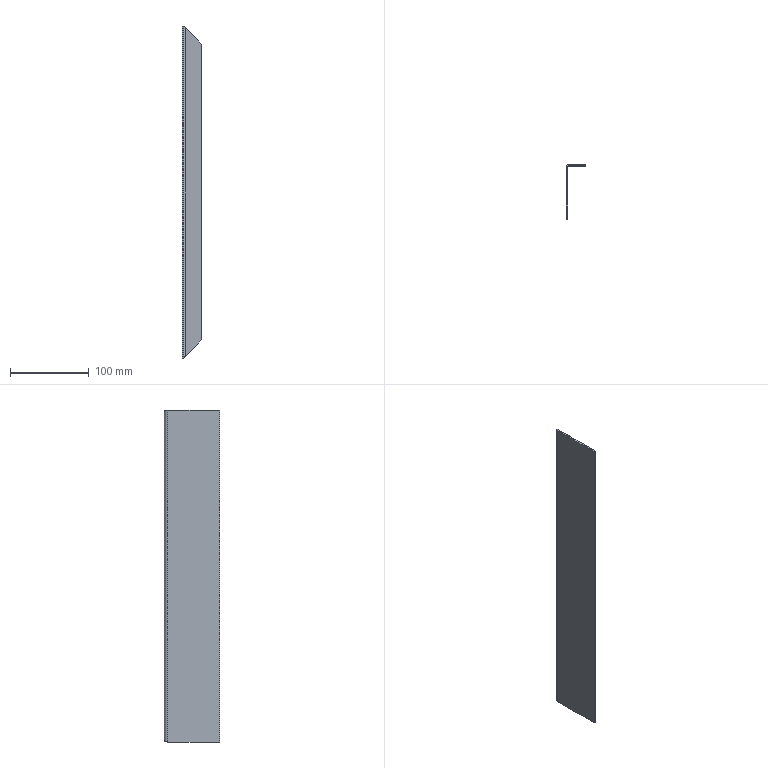Part | STEP file | 750038405 | 1 solid | 14 faces | box 25 x 70 x 422 mm | volume 76342 mm3 | plane 10 | cylinder 2 | spline 2 | commonest cylinder face diameters 4 x1 8 x1
STEP:
#1=CARTESIAN_POINT('',(0.,66.,-211.));
#2=VERTEX_POINT('',#1);
#3=CARTESIAN_POINT('',(0.,0.,-211.));
#4=VERTEX_POINT('',#3);
#5=CARTESIAN_POINT('',(0.,0.,-211.));
#6=DIRECTION('',(0.,-1.,0.));
#7=VECTOR('',#6,1000.);
#8=LINE('',#5,#7);
#9=EDGE_CURVE('',#2,#4,#8,.T.);
#10=ORIENTED_EDGE('',*,*,#9,.T.);
#11=CARTESIAN_POINT('',(0.,0.,211.));
#12=VERTEX_POINT('',#11);
#13=CARTESIAN_POINT('',(0.,0.,213.));
#14=DIRECTION('',(0.,0.,1.));
#15=VECTOR('',#14,1000.);
#16=LINE('',#13,#15);
#17=EDGE_CURVE('',#4,#12,#16,.T.);
#18=ORIENTED_EDGE('',*,*,#17,.T.);
#19=CARTESIAN_POINT('',(0.,66.,211.));
#20=VERTEX_POINT('',#19);
#21=CARTESIAN_POINT('',(0.,0.,211.));
#22=DIRECTION('',(0.,1.,0.));
#23=VECTOR('',#22,1000.);
#24=LINE('',#21,#23);
#25=EDGE_CURVE('',#12,#20,#24,.T.);
#26=ORIENTED_EDGE('',*,*,#25,.T.);
#27=CARTESIAN_POINT('',(0.,66.,213.));
#28=DIRECTION('',(0.,0.,-1.));
#29=VECTOR('',#28,1000.);
#30=LINE('',#27,#29);
#31=EDGE_CURVE('',#20,#2,#30,.T.);
#32=ORIENTED_EDGE('',*,*,#31,.T.);
#33=EDGE_LOOP('',(#10,#18,#26,#32));
#34=FACE_OUTER_BOUND('',#33,.T.);
#35=CARTESIAN_POINT('',(0.,0.,213.));
#36=DIRECTION('',(-1.,0.,0.));
#37=DIRECTION('',(0.,0.,1.));
#38=AXIS2_PLACEMENT_3D('',#35,#36,#37);
#39=PLANE('',#38);
#40=ADVANCED_FACE('',(#34),#39,.T.);
#41=ORIENTED_EDGE('',*,*,#17,.F.);
#42=CARTESIAN_POINT('',(2.,0.,-211.));
#43=VERTEX_POINT('',#42);
#44=CARTESIAN_POINT('',(0.,0.,-211.));
#45=DIRECTION('',(-1.,0.,0.));
#46=VECTOR('',#45,1000.);
#47=LINE('',#44,#46);
#48=EDGE_CURVE('',#43,#4,#47,.T.);
#49=ORIENTED_EDGE('',*,*,#48,.F.);
#50=CARTESIAN_POINT('',(2.,0.,211.));
#51=VERTEX_POINT('',#50);
#52=CARTESIAN_POINT('',(2.,0.,213.));
#53=DIRECTION('',(0.,0.,-1.));
#54=VECTOR('',#53,1000.);
#55=LINE('',#52,#54);
#56=EDGE_CURVE('',#51,#43,#55,.T.);
#57=ORIENTED_EDGE('',*,*,#56,.F.);
#58=CARTESIAN_POINT('',(0.,0.,211.));
#59=DIRECTION('',(1.,0.,0.));
#60=VECTOR('',#59,1000.);
#61=LINE('',#58,#60);
#62=EDGE_CURVE('',#12,#51,#61,.T.);
#63=ORIENTED_EDGE('',*,*,#62,.F.);
#64=EDGE_LOOP('',(#41,#49,#57,#63));
#65=FACE_OUTER_BOUND('',#64,.T.);
#66=CARTESIAN_POINT('',(0.,0.,213.));
#67=DIRECTION('',(0.,1.,0.));
#68=DIRECTION('',(0.,0.,1.));
#69=AXIS2_PLACEMENT_3D('',#66,#67,#68);
#70=PLANE('',#69);
#71=ADVANCED_FACE('',(#65),#70,.F.);
#72=CARTESIAN_POINT('',(2.,66.,-211.));
#73=VERTEX_POINT('',#72);
#74=CARTESIAN_POINT('',(2.,66.,-211.));
#75=DIRECTION('',(-1.,0.,0.));
#76=VECTOR('',#75,1000.);
#77=LINE('',#74,#76);
#78=EDGE_CURVE('',#73,#2,#77,.T.);
#79=ORIENTED_EDGE('',*,*,#78,.F.);
#80=CARTESIAN_POINT('',(2.,0.,-211.));
#81=DIRECTION('',(0.,1.,0.));
#82=VECTOR('',#81,1000.);
#83=LINE('',#80,#82);
#84=EDGE_CURVE('',#43,#73,#83,.T.);
#85=ORIENTED_EDGE('',*,*,#84,.F.);
#86=ORIENTED_EDGE('',*,*,#48,.T.);
#87=ORIENTED_EDGE('',*,*,#9,.F.);
#88=EDGE_LOOP('',(#79,#85,#86,#87));
#89=FACE_OUTER_BOUND('',#88,.T.);
#90=CARTESIAN_POINT('',(2.,0.,-211.));
#91=DIRECTION('',(0.,0.,1.));
#92=DIRECTION('',(1.,0.,0.));
#93=AXIS2_PLACEMENT_3D('',#90,#91,#92);
#94=PLANE('',#93);
#95=ADVANCED_FACE('',(#89),#94,.F.);
#96=CARTESIAN_POINT('',(4.,70.,-209.));
#97=VERTEX_POINT('',#96);
#98=CARTESIAN_POINT('',(4.,70.,-209.));
#99=CARTESIAN_POINT('',(1.333,70.,-210.333));
#100=CARTESIAN_POINT('',(0.,68.,-211.));
#101=CARTESIAN_POINT('',(0.,66.,-211.));
#102=(BOUNDED_CURVE()B_SPLINE_CURVE(3,(#98,#99,#100,#101),.UNSPECIFIED.,.F.,.F.)B_SPLINE_CURVE_WITH_KNOTS((4,4),(0.,0.006641),.UNSPECIFIED.)CURVE()GEOMETRIC_REPRESENTATION_ITEM()RATIONAL_B_SPLINE_CURVE((0.5,0.5,0.6667,1.))REPRESENTATION_ITEM(''));
#103=EDGE_CURVE('',#97,#2,#102,.T.);
#104=ORIENTED_EDGE('',*,*,#103,.T.);
#105=ORIENTED_EDGE('',*,*,#31,.F.);
#106=CARTESIAN_POINT('',(4.,70.,209.));
#107=VERTEX_POINT('',#106);
#108=CARTESIAN_POINT('',(0.,66.,211.));
#109=CARTESIAN_POINT('',(0.,68.,211.));
#110=CARTESIAN_POINT('',(1.333,70.,210.333));
#111=CARTESIAN_POINT('',(4.,70.,209.));
#112=(BOUNDED_CURVE()B_SPLINE_CURVE(3,(#108,#109,#110,#111),.UNSPECIFIED.,.F.,.F.)B_SPLINE_CURVE_WITH_KNOTS((4,4),(0.,0.006627),.UNSPECIFIED.)CURVE()GEOMETRIC_REPRESENTATION_ITEM()RATIONAL_B_SPLINE_CURVE((1.,0.6667,0.5,0.5))REPRESENTATION_ITEM(''));
#113=EDGE_CURVE('',#20,#107,#112,.T.);
#114=ORIENTED_EDGE('',*,*,#113,.T.);
#115=CARTESIAN_POINT('',(4.,70.,213.));
#116=DIRECTION('',(0.,0.,-1.));
#117=VECTOR('',#116,1000.);
#118=LINE('',#115,#117);
#119=EDGE_CURVE('',#107,#97,#118,.T.);
#120=ORIENTED_EDGE('',*,*,#119,.T.);
#121=EDGE_LOOP('',(#104,#105,#114,#120));
#122=FACE_OUTER_BOUND('',#121,.T.);
#123=CARTESIAN_POINT('',(4.,66.,213.));
#124=DIRECTION('',(0.,0.,-1.));
#125=DIRECTION('',(-1.,0.,0.));
#126=AXIS2_PLACEMENT_3D('',#123,#124,#125);
#127=CYLINDRICAL_SURFACE('',#126,4.);
#128=ADVANCED_FACE('',(#122),#127,.T.);
#129=CARTESIAN_POINT('',(2.,66.,211.));
#130=VERTEX_POINT('',#129);
#131=CARTESIAN_POINT('',(2.,0.,211.));
#132=DIRECTION('',(0.,-1.,0.));
#133=VECTOR('',#132,1000.);
#134=LINE('',#131,#133);
#135=EDGE_CURVE('',#130,#51,#134,.T.);
#136=ORIENTED_EDGE('',*,*,#135,.F.);
#137=CARTESIAN_POINT('',(2.,66.,211.));
#138=DIRECTION('',(1.,0.,0.));
#139=VECTOR('',#138,1000.);
#140=LINE('',#137,#139);
#141=EDGE_CURVE('',#20,#130,#140,.T.);
#142=ORIENTED_EDGE('',*,*,#141,.F.);
#143=ORIENTED_EDGE('',*,*,#25,.F.);
#144=ORIENTED_EDGE('',*,*,#62,.T.);
#145=EDGE_LOOP('',(#136,#142,#143,#144));
#146=FACE_OUTER_BOUND('',#145,.T.);
#147=CARTESIAN_POINT('',(2.,0.,211.));
#148=DIRECTION('',(0.,0.,-1.));
#149=DIRECTION('',(-1.,0.,0.));
#150=AXIS2_PLACEMENT_3D('',#147,#148,#149);
#151=PLANE('',#150);
#152=ADVANCED_FACE('',(#146),#151,.F.);
#153=ORIENTED_EDGE('',*,*,#135,.T.);
#154=ORIENTED_EDGE('',*,*,#56,.T.);
#155=ORIENTED_EDGE('',*,*,#84,.T.);
#156=CARTESIAN_POINT('',(2.,66.,213.));
#157=DIRECTION('',(0.,0.,-1.));
#158=VECTOR('',#157,1000.);
#159=LINE('',#156,#158);
#160=EDGE_CURVE('',#130,#73,#159,.T.);
#161=ORIENTED_EDGE('',*,*,#160,.F.);
#162=EDGE_LOOP('',(#153,#154,#155,#161));
#163=FACE_OUTER_BOUND('',#162,.T.);
#164=CARTESIAN_POINT('',(2.,0.,213.));
#165=DIRECTION('',(-1.,0.,0.));
#166=DIRECTION('',(0.,0.,1.));
#167=AXIS2_PLACEMENT_3D('',#164,#165,#166);
#168=PLANE('',#167);
#169=ADVANCED_FACE('',(#163),#168,.F.);
#170=ORIENTED_EDGE('',*,*,#78,.T.);
#171=ORIENTED_EDGE('',*,*,#103,.F.);
#172=CARTESIAN_POINT('',(4.,68.,-209.));
#173=VERTEX_POINT('',#172);
#174=CARTESIAN_POINT('',(4.,69.,-209.));
#175=DIRECTION('',(0.,-1.,0.));
#176=VECTOR('',#175,1000.);
#177=LINE('',#174,#176);
#178=EDGE_CURVE('',#97,#173,#177,.T.);
#179=ORIENTED_EDGE('',*,*,#178,.T.);
#180=CARTESIAN_POINT('',(4.,68.,-209.));
#181=CARTESIAN_POINT('',(2.667,68.,-210.333));
#182=CARTESIAN_POINT('',(2.,67.,-211.));
#183=CARTESIAN_POINT('',(2.,66.,-211.));
#184=(BOUNDED_CURVE()B_SPLINE_CURVE(3,(#180,#181,#182,#183),.UNSPECIFIED.,.F.,.F.)B_SPLINE_CURVE_WITH_KNOTS((4,4),(0.,0.003785),.UNSPECIFIED.)CURVE()GEOMETRIC_REPRESENTATION_ITEM()RATIONAL_B_SPLINE_CURVE((0.5,0.5,0.6667,1.))REPRESENTATION_ITEM(''));
#185=EDGE_CURVE('',#173,#73,#184,.T.);
#186=ORIENTED_EDGE('',*,*,#185,.T.);
#187=EDGE_LOOP('',(#170,#171,#179,#186));
#188=FACE_OUTER_BOUND('',#187,.T.);
#189=CARTESIAN_POINT('',(0.,66.,-211.));
#190=CARTESIAN_POINT('',(0.6667,66.,-211.));
#191=CARTESIAN_POINT('',(1.333,66.,-211.));
#192=CARTESIAN_POINT('',(2.,66.,-211.));
#193=CARTESIAN_POINT('',(0.,74.,-211.));
#194=CARTESIAN_POINT('',(0.6667,72.667,-211.));
#195=CARTESIAN_POINT('',(1.333,71.333,-211.));
#196=CARTESIAN_POINT('',(2.,70.,-211.));
#197=CARTESIAN_POINT('',(8.,74.,-207.));
#198=CARTESIAN_POINT('',(7.333,72.667,-207.));
#199=CARTESIAN_POINT('',(6.667,71.333,-207.));
#200=CARTESIAN_POINT('',(6.,70.,-207.));
#201=CARTESIAN_POINT('',(8.,66.,-207.));
#202=CARTESIAN_POINT('',(7.333,66.,-207.));
#203=CARTESIAN_POINT('',(6.667,66.,-207.));
#204=CARTESIAN_POINT('',(6.,66.,-207.));
#205=CARTESIAN_POINT('',(8.,58.,-207.));
#206=CARTESIAN_POINT('',(7.333,59.333,-207.));
#207=CARTESIAN_POINT('',(6.667,60.667,-207.));
#208=CARTESIAN_POINT('',(6.,62.,-207.));
#209=CARTESIAN_POINT('',(0.,58.,-211.));
#210=CARTESIAN_POINT('',(0.6667,59.333,-211.));
#211=CARTESIAN_POINT('',(1.333,60.667,-211.));
#212=CARTESIAN_POINT('',(2.,62.,-211.));
#213=CARTESIAN_POINT('',(0.,66.,-211.));
#214=CARTESIAN_POINT('',(0.6667,66.,-211.));
#215=CARTESIAN_POINT('',(1.333,66.,-211.));
#216=CARTESIAN_POINT('',(2.,66.,-211.));
#217=(BOUNDED_SURFACE()B_SPLINE_SURFACE(3,3,((#189,#190,#191,#192),(#193,#194,#195,#196),(#197,#198,#199,#200),(#201,#202,#203,#204),(#205,#206,#207,#208),(#209,#210,#211,#212),(#213,#214,#215,#216)),.UNSPECIFIED.,.T.,.F.,.F.)B_SPLINE_SURFACE_WITH_KNOTS((4,3,4),(4,4),(0.,0.5,1.),(0.,1.),.UNSPECIFIED.)GEOMETRIC_REPRESENTATION_ITEM()RATIONAL_B_SPLINE_SURFACE(((1.,1.,1.,1.),(0.3333,0.3333,0.3333,0.3333),(0.3333,0.3333,0.3333,0.3333),(1.,1.,1.,1.),(0.3333,0.3333,0.3333,0.3333),(0.3333,0.3333,0.3333,0.3333),(1.,1.,1.,1.)))REPRESENTATION_ITEM('')SURFACE());
#218=ADVANCED_FACE('',(#188),#217,.T.);
#219=CARTESIAN_POINT('',(25.,70.,-188.));
#220=VERTEX_POINT('',#219);
#221=CARTESIAN_POINT('',(25.,70.,-188.));
#222=DIRECTION('',(-0.7071,0.,-0.7071));
#223=VECTOR('',#222,1000.);
#224=LINE('',#221,#223);
#225=EDGE_CURVE('',#220,#97,#224,.T.);
#226=ORIENTED_EDGE('',*,*,#225,.T.);
#227=ORIENTED_EDGE('',*,*,#119,.F.);
#228=CARTESIAN_POINT('',(25.,70.,188.));
#229=VERTEX_POINT('',#228);
#230=CARTESIAN_POINT('',(4.,70.,209.));
#231=DIRECTION('',(0.7071,0.,-0.7071));
#232=VECTOR('',#231,1000.);
#233=LINE('',#230,#232);
#234=EDGE_CURVE('',#107,#229,#233,.T.);
#235=ORIENTED_EDGE('',*,*,#234,.T.);
#236=CARTESIAN_POINT('',(25.,70.,213.));
#237=DIRECTION('',(0.,0.,-1.));
#238=VECTOR('',#237,1000.);
#239=LINE('',#236,#238);
#240=EDGE_CURVE('',#229,#220,#239,.T.);
#241=ORIENTED_EDGE('',*,*,#240,.T.);
#242=EDGE_LOOP('',(#226,#227,#235,#241));
#243=FACE_OUTER_BOUND('',#242,.T.);
#244=CARTESIAN_POINT('',(0.,70.,213.));
#245=DIRECTION('',(0.,1.,0.));
#246=DIRECTION('',(0.,0.,1.));
#247=AXIS2_PLACEMENT_3D('',#244,#245,#246);
#248=PLANE('',#247);
#249=ADVANCED_FACE('',(#243),#248,.T.);
#250=CARTESIAN_POINT('',(4.,68.,209.));
#251=VERTEX_POINT('',#250);
#252=CARTESIAN_POINT('',(4.,69.,209.));
#253=DIRECTION('',(0.,1.,0.));
#254=VECTOR('',#253,1000.);
#255=LINE('',#252,#254);
#256=EDGE_CURVE('',#251,#107,#255,.T.);
#257=ORIENTED_EDGE('',*,*,#256,.T.);
#258=ORIENTED_EDGE('',*,*,#113,.F.);
#259=ORIENTED_EDGE('',*,*,#141,.T.);
#260=CARTESIAN_POINT('',(2.,66.,211.));
#261=CARTESIAN_POINT('',(2.,67.,211.));
#262=CARTESIAN_POINT('',(2.667,68.,210.333));
#263=CARTESIAN_POINT('',(4.,68.,209.));
#264=(BOUNDED_CURVE()B_SPLINE_CURVE(3,(#260,#261,#262,#263),.UNSPECIFIED.,.F.,.F.)B_SPLINE_CURVE_WITH_KNOTS((4,4),(0.,0.003806),.UNSPECIFIED.)CURVE()GEOMETRIC_REPRESENTATION_ITEM()RATIONAL_B_SPLINE_CURVE((1.,0.6667,0.5,0.5))REPRESENTATION_ITEM(''));
#265=EDGE_CURVE('',#130,#251,#264,.T.);
#266=ORIENTED_EDGE('',*,*,#265,.T.);
#267=EDGE_LOOP('',(#257,#258,#259,#266));
#268=FACE_OUTER_BOUND('',#267,.T.);
#269=CARTESIAN_POINT('',(8.,66.,207.));
#270=CARTESIAN_POINT('',(7.333,66.,207.));
#271=CARTESIAN_POINT('',(6.667,66.,207.));
#272=CARTESIAN_POINT('',(6.,66.,207.));
#273=CARTESIAN_POINT('',(8.,74.,207.));
#274=CARTESIAN_POINT('',(7.333,72.667,207.));
#275=CARTESIAN_POINT('',(6.667,71.333,207.));
#276=CARTESIAN_POINT('',(6.,70.,207.));
#277=CARTESIAN_POINT('',(0.,74.,211.));
#278=CARTESIAN_POINT('',(0.6667,72.667,211.));
#279=CARTESIAN_POINT('',(1.333,71.333,211.));
#280=CARTESIAN_POINT('',(2.,70.,211.));
#281=CARTESIAN_POINT('',(0.,66.,211.));
#282=CARTESIAN_POINT('',(0.6667,66.,211.));
#283=CARTESIAN_POINT('',(1.333,66.,211.));
#284=CARTESIAN_POINT('',(2.,66.,211.));
#285=CARTESIAN_POINT('',(0.,58.,211.));
#286=CARTESIAN_POINT('',(0.6667,59.333,211.));
#287=CARTESIAN_POINT('',(1.333,60.667,211.));
#288=CARTESIAN_POINT('',(2.,62.,211.));
#289=CARTESIAN_POINT('',(8.,58.,207.));
#290=CARTESIAN_POINT('',(7.333,59.333,207.));
#291=CARTESIAN_POINT('',(6.667,60.667,207.));
#292=CARTESIAN_POINT('',(6.,62.,207.));
#293=CARTESIAN_POINT('',(8.,66.,207.));
#294=CARTESIAN_POINT('',(7.333,66.,207.));
#295=CARTESIAN_POINT('',(6.667,66.,207.));
#296=CARTESIAN_POINT('',(6.,66.,207.));
#297=(BOUNDED_SURFACE()B_SPLINE_SURFACE(3,3,((#269,#270,#271,#272),(#273,#274,#275,#276),(#277,#278,#279,#280),(#281,#282,#283,#284),(#285,#286,#287,#288),(#289,#290,#291,#292),(#293,#294,#295,#296)),.UNSPECIFIED.,.T.,.F.,.F.)B_SPLINE_SURFACE_WITH_KNOTS((4,3,4),(4,4),(0.,0.5,1.),(0.,1.),.UNSPECIFIED.)GEOMETRIC_REPRESENTATION_ITEM()RATIONAL_B_SPLINE_SURFACE(((1.,1.,1.,1.),(0.3333,0.3333,0.3333,0.3333),(0.3333,0.3333,0.3333,0.3333),(1.,1.,1.,1.),(0.3333,0.3333,0.3333,0.3333),(0.3333,0.3333,0.3333,0.3333),(1.,1.,1.,1.)))REPRESENTATION_ITEM('')SURFACE());
#298=ADVANCED_FACE('',(#268),#297,.T.);
#299=ORIENTED_EDGE('',*,*,#265,.F.);
#300=ORIENTED_EDGE('',*,*,#160,.T.);
#301=ORIENTED_EDGE('',*,*,#185,.F.);
#302=CARTESIAN_POINT('',(4.,68.,213.));
#303=DIRECTION('',(0.,0.,-1.));
#304=VECTOR('',#303,1000.);
#305=LINE('',#302,#304);
#306=EDGE_CURVE('',#251,#173,#305,.T.);
#307=ORIENTED_EDGE('',*,*,#306,.F.);
#308=EDGE_LOOP('',(#299,#300,#301,#307));
#309=FACE_OUTER_BOUND('',#308,.T.);
#310=CARTESIAN_POINT('',(4.,66.,213.));
#311=DIRECTION('',(0.,0.,-1.));
#312=DIRECTION('',(-1.,0.,0.));
#313=AXIS2_PLACEMENT_3D('',#310,#311,#312);
#314=CYLINDRICAL_SURFACE('',#313,2.);
#315=ADVANCED_FACE('',(#309),#314,.F.);
#316=ORIENTED_EDGE('',*,*,#225,.F.);
#317=CARTESIAN_POINT('',(25.,68.,-188.));
#318=VERTEX_POINT('',#317);
#319=CARTESIAN_POINT('',(25.,70.,-188.));
#320=DIRECTION('',(0.,1.,0.));
#321=VECTOR('',#320,1000.);
#322=LINE('',#319,#321);
#323=EDGE_CURVE('',#318,#220,#322,.T.);
#324=ORIENTED_EDGE('',*,*,#323,.F.);
#325=CARTESIAN_POINT('',(213.,68.,0.));
#326=DIRECTION('',(0.7071,0.,0.7071));
#327=VECTOR('',#326,1000.);
#328=LINE('',#325,#327);
#329=EDGE_CURVE('',#173,#318,#328,.T.);
#330=ORIENTED_EDGE('',*,*,#329,.F.);
#331=ORIENTED_EDGE('',*,*,#178,.F.);
#332=EDGE_LOOP('',(#316,#324,#330,#331));
#333=FACE_OUTER_BOUND('',#332,.T.);
#334=CARTESIAN_POINT('',(213.,70.,0.));
#335=DIRECTION('',(-0.7071,0.,0.7071));
#336=DIRECTION('',(0.7071,0.,0.7071));
#337=AXIS2_PLACEMENT_3D('',#334,#335,#336);
#338=PLANE('',#337);
#339=ADVANCED_FACE('',(#333),#338,.F.);
#340=ORIENTED_EDGE('',*,*,#323,.T.);
#341=ORIENTED_EDGE('',*,*,#240,.F.);
#342=CARTESIAN_POINT('',(25.,68.,188.));
#343=VERTEX_POINT('',#342);
#344=CARTESIAN_POINT('',(25.,70.,188.));
#345=DIRECTION('',(0.,-1.,0.));
#346=VECTOR('',#345,1000.);
#347=LINE('',#344,#346);
#348=EDGE_CURVE('',#229,#343,#347,.T.);
#349=ORIENTED_EDGE('',*,*,#348,.T.);
#350=CARTESIAN_POINT('',(25.,68.,213.));
#351=DIRECTION('',(0.,0.,-1.));
#352=VECTOR('',#351,1000.);
#353=LINE('',#350,#352);
#354=EDGE_CURVE('',#343,#318,#353,.T.);
#355=ORIENTED_EDGE('',*,*,#354,.T.);
#356=EDGE_LOOP('',(#340,#341,#349,#355));
#357=FACE_OUTER_BOUND('',#356,.T.);
#358=CARTESIAN_POINT('',(25.,70.,213.));
#359=DIRECTION('',(1.,0.,0.));
#360=DIRECTION('',(0.,0.,-1.));
#361=AXIS2_PLACEMENT_3D('',#358,#359,#360);
#362=PLANE('',#361);
#363=ADVANCED_FACE('',(#357),#362,.T.);
#364=ORIENTED_EDGE('',*,*,#234,.F.);
#365=ORIENTED_EDGE('',*,*,#256,.F.);
#366=CARTESIAN_POINT('',(0.,68.,213.));
#367=DIRECTION('',(-0.7071,0.,0.7071));
#368=VECTOR('',#367,1000.);
#369=LINE('',#366,#368);
#370=EDGE_CURVE('',#343,#251,#369,.T.);
#371=ORIENTED_EDGE('',*,*,#370,.F.);
#372=ORIENTED_EDGE('',*,*,#348,.F.);
#373=EDGE_LOOP('',(#364,#365,#371,#372));
#374=FACE_OUTER_BOUND('',#373,.T.);
#375=CARTESIAN_POINT('',(0.,70.,213.));
#376=DIRECTION('',(-0.7071,0.,-0.7071));
#377=DIRECTION('',(-0.7071,0.,0.7071));
#378=AXIS2_PLACEMENT_3D('',#375,#376,#377);
#379=PLANE('',#378);
#380=ADVANCED_FACE('',(#374),#379,.F.);
#381=ORIENTED_EDGE('',*,*,#370,.T.);
#382=ORIENTED_EDGE('',*,*,#306,.T.);
#383=ORIENTED_EDGE('',*,*,#329,.T.);
#384=ORIENTED_EDGE('',*,*,#354,.F.);
#385=EDGE_LOOP('',(#381,#382,#383,#384));
#386=FACE_OUTER_BOUND('',#385,.T.);
#387=CARTESIAN_POINT('',(0.,68.,213.));
#388=DIRECTION('',(0.,1.,0.));
#389=DIRECTION('',(0.,0.,1.));
#390=AXIS2_PLACEMENT_3D('',#387,#388,#389);
#391=PLANE('',#390);
#392=ADVANCED_FACE('',(#386),#391,.F.);
#393=CLOSED_SHELL('',(#40,#71,#95,#128,#152,#169,#218,#249,#298,#315,#339,#363,#380,#392));
#394=MANIFOLD_SOLID_BREP('',#393);
#395=CARTESIAN_POINT('',(0.,0.,0.));
#396=DIRECTION('',(0.,0.,1.));
#397=DIRECTION('',(1.,0.,0.));
#398=AXIS2_PLACEMENT_3D('',#395,#396,#397);
#399=(LENGTH_UNIT()NAMED_UNIT(*)SI_UNIT(.MILLI.,.METRE.));
#400=UNCERTAINTY_MEASURE_WITH_UNIT(LENGTH_MEASURE(0.00001),#399,'','');
#401=(NAMED_UNIT(*)PLANE_ANGLE_UNIT()SI_UNIT($,.RADIAN.));
#402=(NAMED_UNIT(*)SI_UNIT($,.STERADIAN.)SOLID_ANGLE_UNIT());
#403=(GEOMETRIC_REPRESENTATION_CONTEXT(3)GLOBAL_UNCERTAINTY_ASSIGNED_CONTEXT((#400))GLOBAL_UNIT_ASSIGNED_CONTEXT((#399,#401,#402))REPRESENTATION_CONTEXT('',''));
#404=ADVANCED_BREP_SHAPE_REPRESENTATION('',(#394,#398),#403);